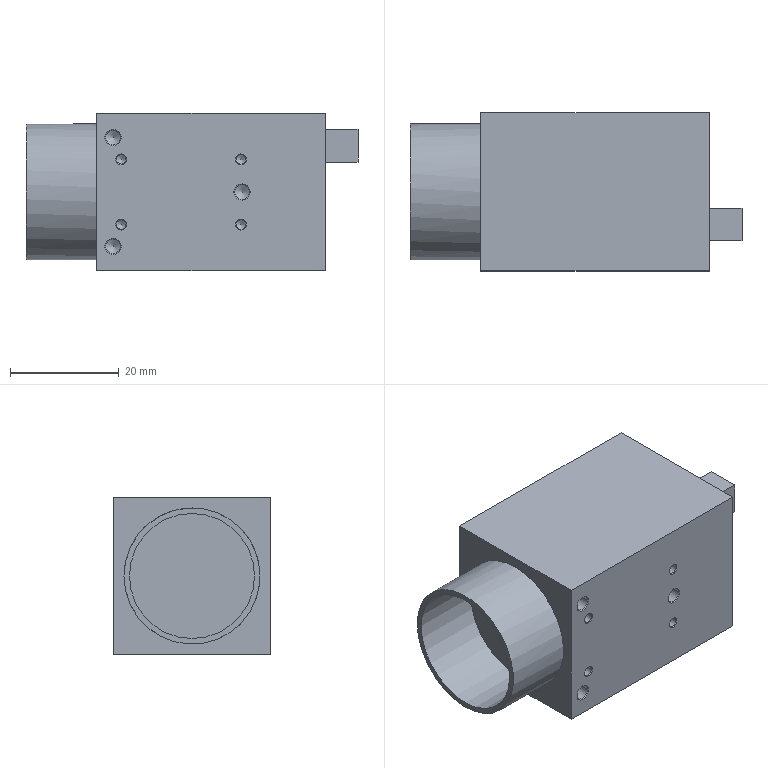Part | NX | features SIMPLE HOLE 7, SYMBOLIC_THREAD 7, DATUM_CSYS 6, SKETCH 5, EXTRUDE 4, HOLE PACKAGE 2 | 1 solid | 36 faces | box 61 x 29 x 29 mm | volume 36377 mm3 | cone 14 | plane 13 | cylinder 9 | commonest cylinder face diameters 1.75 x4 2.7 x3 23 x1 25 x1
STEP:
#1=CARTESIAN_POINT('',(16.,-14.5,-8.5));
#2=VERTEX_POINT('',#1);
#3=CARTESIAN_POINT('',(16.,-14.5,-10.));
#4=DIRECTION('',(0.,1.,0.));
#5=DIRECTION('',(0.,0.,1.));
#6=AXIS2_PLACEMENT_3D('',#3,#4,#5);
#7=CIRCLE('',#6,1.5);
#8=EDGE_CURVE('',#2,#2,#7,.T.);
#9=ORIENTED_EDGE('',*,*,#8,.T.);
#10=EDGE_LOOP('',(#9));
#11=FACE_BOUND('',#10,.T.);
#12=CARTESIAN_POINT('',(16.,-14.5,11.5));
#13=VERTEX_POINT('',#12);
#14=CARTESIAN_POINT('',(16.,-14.5,10.));
#15=DIRECTION('',(0.,1.,0.));
#16=DIRECTION('',(0.,0.,1.));
#17=AXIS2_PLACEMENT_3D('',#14,#15,#16);
#18=CIRCLE('',#17,1.5);
#19=EDGE_CURVE('',#13,#13,#18,.T.);
#20=ORIENTED_EDGE('',*,*,#19,.T.);
#21=EDGE_LOOP('',(#20));
#22=FACE_BOUND('',#21,.T.);
#23=CARTESIAN_POINT('',(39.7,-14.5,1.5));
#24=VERTEX_POINT('',#23);
#25=CARTESIAN_POINT('',(39.7,-14.5,0.));
#26=DIRECTION('',(0.,1.,0.));
#27=DIRECTION('',(0.,0.,1.));
#28=AXIS2_PLACEMENT_3D('',#25,#26,#27);
#29=CIRCLE('',#28,1.5);
#30=EDGE_CURVE('',#24,#24,#29,.T.);
#31=ORIENTED_EDGE('',*,*,#30,.T.);
#32=EDGE_LOOP('',(#31));
#33=FACE_BOUND('',#32,.T.);
#34=CARTESIAN_POINT('',(39.5,-14.5,-5.));
#35=VERTEX_POINT('',#34);
#36=CARTESIAN_POINT('',(39.5,-14.5,-6.));
#37=DIRECTION('',(0.,1.,0.));
#38=DIRECTION('',(0.,0.,1.));
#39=AXIS2_PLACEMENT_3D('',#36,#37,#38);
#40=CIRCLE('',#39,1.);
#41=EDGE_CURVE('',#35,#35,#40,.T.);
#42=ORIENTED_EDGE('',*,*,#41,.T.);
#43=EDGE_LOOP('',(#42));
#44=FACE_BOUND('',#43,.T.);
#45=CARTESIAN_POINT('',(39.5,-14.5,7.));
#46=VERTEX_POINT('',#45);
#47=CARTESIAN_POINT('',(39.5,-14.5,6.));
#48=DIRECTION('',(0.,1.,0.));
#49=DIRECTION('',(0.,0.,1.));
#50=AXIS2_PLACEMENT_3D('',#47,#48,#49);
#51=CIRCLE('',#50,1.);
#52=EDGE_CURVE('',#46,#46,#51,.T.);
#53=ORIENTED_EDGE('',*,*,#52,.T.);
#54=EDGE_LOOP('',(#53));
#55=FACE_BOUND('',#54,.T.);
#56=CARTESIAN_POINT('',(17.5,-14.5,-5.));
#57=VERTEX_POINT('',#56);
#58=CARTESIAN_POINT('',(17.5,-14.5,-6.));
#59=DIRECTION('',(0.,1.,0.));
#60=DIRECTION('',(0.,0.,1.));
#61=AXIS2_PLACEMENT_3D('',#58,#59,#60);
#62=CIRCLE('',#61,1.);
#63=EDGE_CURVE('',#57,#57,#62,.T.);
#64=ORIENTED_EDGE('',*,*,#63,.T.);
#65=EDGE_LOOP('',(#64));
#66=FACE_BOUND('',#65,.T.);
#67=CARTESIAN_POINT('',(17.5,-14.5,7.));
#68=VERTEX_POINT('',#67);
#69=CARTESIAN_POINT('',(17.5,-14.5,6.));
#70=DIRECTION('',(0.,1.,0.));
#71=DIRECTION('',(0.,0.,1.));
#72=AXIS2_PLACEMENT_3D('',#69,#70,#71);
#73=CIRCLE('',#72,1.);
#74=EDGE_CURVE('',#68,#68,#73,.T.);
#75=ORIENTED_EDGE('',*,*,#74,.T.);
#76=EDGE_LOOP('',(#75));
#77=FACE_BOUND('',#76,.T.);
#78=CARTESIAN_POINT('',(13.,-14.5,-14.5));
#79=VERTEX_POINT('',#78);
#80=CARTESIAN_POINT('',(13.,-14.5,14.5));
#81=VERTEX_POINT('',#80);
#82=CARTESIAN_POINT('',(13.,-14.5,-14.5));
#83=DIRECTION('',(0.,0.,1.));
#84=VECTOR('',#83,1000.);
#85=LINE('',#82,#84);
#86=EDGE_CURVE('',#79,#81,#85,.T.);
#87=ORIENTED_EDGE('',*,*,#86,.F.);
#88=CARTESIAN_POINT('',(55.,-14.5,-14.5));
#89=VERTEX_POINT('',#88);
#90=CARTESIAN_POINT('',(55.,-14.5,-14.5));
#91=DIRECTION('',(-1.,0.,0.));
#92=VECTOR('',#91,1000.);
#93=LINE('',#90,#92);
#94=EDGE_CURVE('',#89,#79,#93,.T.);
#95=ORIENTED_EDGE('',*,*,#94,.F.);
#96=CARTESIAN_POINT('',(55.,-14.5,14.5));
#97=VERTEX_POINT('',#96);
#98=CARTESIAN_POINT('',(55.,-14.5,14.5));
#99=DIRECTION('',(0.,0.,-1.));
#100=VECTOR('',#99,1000.);
#101=LINE('',#98,#100);
#102=EDGE_CURVE('',#97,#89,#101,.T.);
#103=ORIENTED_EDGE('',*,*,#102,.F.);
#104=CARTESIAN_POINT('',(55.,-14.5,14.5));
#105=DIRECTION('',(-1.,0.,0.));
#106=VECTOR('',#105,1000.);
#107=LINE('',#104,#106);
#108=EDGE_CURVE('',#97,#81,#107,.T.);
#109=ORIENTED_EDGE('',*,*,#108,.T.);
#110=EDGE_LOOP('',(#87,#95,#103,#109));
#111=FACE_BOUND('',#110,.T.);
#112=CARTESIAN_POINT('',(55.,-14.5,14.5));
#113=DIRECTION('',(0.,1.,0.));
#114=DIRECTION('',(0.,0.,1.));
#115=AXIS2_PLACEMENT_3D('',#112,#113,#114);
#116=PLANE('',#115);
#117=ADVANCED_FACE('',(#11,#22,#33,#44,#55,#66,#77,#111),#116,.F.);
#118=CARTESIAN_POINT('',(13.,14.5,-14.5));
#119=VERTEX_POINT('',#118);
#120=CARTESIAN_POINT('',(13.,14.5,-14.5));
#121=DIRECTION('',(0.,-1.,0.));
#122=VECTOR('',#121,1000.);
#123=LINE('',#120,#122);
#124=EDGE_CURVE('',#119,#79,#123,.T.);
#125=ORIENTED_EDGE('',*,*,#124,.F.);
#126=CARTESIAN_POINT('',(55.,14.5,-14.5));
#127=VERTEX_POINT('',#126);
#128=CARTESIAN_POINT('',(55.,14.5,-14.5));
#129=DIRECTION('',(-1.,0.,0.));
#130=VECTOR('',#129,1000.);
#131=LINE('',#128,#130);
#132=EDGE_CURVE('',#127,#119,#131,.T.);
#133=ORIENTED_EDGE('',*,*,#132,.F.);
#134=CARTESIAN_POINT('',(55.,-14.5,-14.5));
#135=DIRECTION('',(0.,1.,0.));
#136=VECTOR('',#135,1000.);
#137=LINE('',#134,#136);
#138=EDGE_CURVE('',#89,#127,#137,.T.);
#139=ORIENTED_EDGE('',*,*,#138,.F.);
#140=ORIENTED_EDGE('',*,*,#94,.T.);
#141=EDGE_LOOP('',(#125,#133,#139,#140));
#142=FACE_BOUND('',#141,.T.);
#143=CARTESIAN_POINT('',(55.,-14.5,-14.5));
#144=DIRECTION('',(0.,0.,1.));
#145=DIRECTION('',(1.,0.,0.));
#146=AXIS2_PLACEMENT_3D('',#143,#144,#145);
#147=PLANE('',#146);
#148=ADVANCED_FACE('',(#142),#147,.F.);
#149=CARTESIAN_POINT('',(13.,14.5,14.5));
#150=VERTEX_POINT('',#149);
#151=CARTESIAN_POINT('',(13.,14.5,14.5));
#152=DIRECTION('',(0.,0.,-1.));
#153=VECTOR('',#152,1000.);
#154=LINE('',#151,#153);
#155=EDGE_CURVE('',#150,#119,#154,.T.);
#156=ORIENTED_EDGE('',*,*,#155,.F.);
#157=CARTESIAN_POINT('',(55.,14.5,14.5));
#158=VERTEX_POINT('',#157);
#159=CARTESIAN_POINT('',(55.,14.5,14.5));
#160=DIRECTION('',(-1.,0.,0.));
#161=VECTOR('',#160,1000.);
#162=LINE('',#159,#161);
#163=EDGE_CURVE('',#158,#150,#162,.T.);
#164=ORIENTED_EDGE('',*,*,#163,.F.);
#165=CARTESIAN_POINT('',(55.,14.5,-14.5));
#166=DIRECTION('',(0.,0.,1.));
#167=VECTOR('',#166,1000.);
#168=LINE('',#165,#167);
#169=EDGE_CURVE('',#127,#158,#168,.T.);
#170=ORIENTED_EDGE('',*,*,#169,.F.);
#171=ORIENTED_EDGE('',*,*,#132,.T.);
#172=EDGE_LOOP('',(#156,#164,#170,#171));
#173=FACE_BOUND('',#172,.T.);
#174=CARTESIAN_POINT('',(55.,14.5,-14.5));
#175=DIRECTION('',(0.,-1.,0.));
#176=DIRECTION('',(0.,0.,-1.));
#177=AXIS2_PLACEMENT_3D('',#174,#175,#176);
#178=PLANE('',#177);
#179=ADVANCED_FACE('',(#173),#178,.F.);
#180=CARTESIAN_POINT('',(13.,-14.5,14.5));
#181=DIRECTION('',(0.,1.,0.));
#182=VECTOR('',#181,1000.);
#183=LINE('',#180,#182);
#184=EDGE_CURVE('',#81,#150,#183,.T.);
#185=ORIENTED_EDGE('',*,*,#184,.F.);
#186=ORIENTED_EDGE('',*,*,#108,.F.);
#187=CARTESIAN_POINT('',(55.,14.5,14.5));
#188=DIRECTION('',(0.,-1.,0.));
#189=VECTOR('',#188,1000.);
#190=LINE('',#187,#189);
#191=EDGE_CURVE('',#158,#97,#190,.T.);
#192=ORIENTED_EDGE('',*,*,#191,.F.);
#193=ORIENTED_EDGE('',*,*,#163,.T.);
#194=EDGE_LOOP('',(#185,#186,#192,#193));
#195=FACE_BOUND('',#194,.T.);
#196=CARTESIAN_POINT('',(55.,14.5,14.5));
#197=DIRECTION('',(0.,0.,-1.));
#198=DIRECTION('',(-1.,0.,0.));
#199=AXIS2_PLACEMENT_3D('',#196,#197,#198);
#200=PLANE('',#199);
#201=ADVANCED_FACE('',(#195),#200,.F.);
#202=CARTESIAN_POINT('',(55.,-9.,11.5));
#203=VERTEX_POINT('',#202);
#204=CARTESIAN_POINT('',(55.,-9.,5.5));
#205=VERTEX_POINT('',#204);
#206=CARTESIAN_POINT('',(55.,-9.,11.5));
#207=DIRECTION('',(0.,0.,-1.));
#208=VECTOR('',#207,1000.);
#209=LINE('',#206,#208);
#210=EDGE_CURVE('',#203,#205,#209,.T.);
#211=ORIENTED_EDGE('',*,*,#210,.F.);
#212=CARTESIAN_POINT('',(55.,-3.,11.5));
#213=VERTEX_POINT('',#212);
#214=CARTESIAN_POINT('',(55.,-3.,11.5));
#215=DIRECTION('',(0.,-1.,0.));
#216=VECTOR('',#215,1000.);
#217=LINE('',#214,#216);
#218=EDGE_CURVE('',#213,#203,#217,.T.);
#219=ORIENTED_EDGE('',*,*,#218,.F.);
#220=CARTESIAN_POINT('',(55.,-3.,5.5));
#221=VERTEX_POINT('',#220);
#222=CARTESIAN_POINT('',(55.,-3.,5.5));
#223=DIRECTION('',(0.,0.,1.));
#224=VECTOR('',#223,1000.);
#225=LINE('',#222,#224);
#226=EDGE_CURVE('',#221,#213,#225,.T.);
#227=ORIENTED_EDGE('',*,*,#226,.F.);
#228=CARTESIAN_POINT('',(55.,-9.,5.5));
#229=DIRECTION('',(0.,1.,0.));
#230=VECTOR('',#229,1000.);
#231=LINE('',#228,#230);
#232=EDGE_CURVE('',#205,#221,#231,.T.);
#233=ORIENTED_EDGE('',*,*,#232,.F.);
#234=EDGE_LOOP('',(#211,#219,#227,#233));
#235=FACE_BOUND('',#234,.T.);
#236=ORIENTED_EDGE('',*,*,#102,.T.);
#237=ORIENTED_EDGE('',*,*,#138,.T.);
#238=ORIENTED_EDGE('',*,*,#169,.T.);
#239=ORIENTED_EDGE('',*,*,#191,.T.);
#240=EDGE_LOOP('',(#236,#237,#238,#239));
#241=FACE_BOUND('',#240,.T.);
#242=CARTESIAN_POINT('',(55.,0.,0.));
#243=DIRECTION('',(1.,0.,0.));
#244=DIRECTION('',(0.,0.,-1.));
#245=AXIS2_PLACEMENT_3D('',#242,#243,#244);
#246=PLANE('',#245);
#247=ADVANCED_FACE('',(#235,#241),#246,.T.);
#248=CARTESIAN_POINT('',(16.,-9.5,-8.65));
#249=VERTEX_POINT('',#248);
#250=CARTESIAN_POINT('',(16.,-9.5,-10.));
#251=DIRECTION('',(0.,1.,0.));
#252=DIRECTION('',(0.,0.,1.));
#253=AXIS2_PLACEMENT_3D('',#250,#251,#252);
#254=CIRCLE('',#253,1.35);
#255=EDGE_CURVE('',#249,#249,#254,.F.);
#256=ORIENTED_EDGE('',*,*,#255,.T.);
#257=EDGE_LOOP('',(#256));
#258=FACE_BOUND('',#257,.T.);
#259=CARTESIAN_POINT('',(16.,-8.689,-10.));
#260=VERTEX_POINT('',#259);
#261=VERTEX_LOOP('',#260);
#262=FACE_BOUND('',#261,.T.);
#263=CARTESIAN_POINT('',(16.,-9.5,-10.));
#264=DIRECTION('',(0.,-1.,0.));
#265=DIRECTION('',(0.,0.,-1.));
#266=AXIS2_PLACEMENT_3D('',#263,#264,#265);
#267=CONICAL_SURFACE('',#266,1.35,1.03);
#268=ADVANCED_FACE('',(#258,#262),#267,.F.);
#269=CARTESIAN_POINT('',(16.,-14.35,-8.65));
#270=VERTEX_POINT('',#269);
#271=CARTESIAN_POINT('',(16.,-14.35,-10.));
#272=DIRECTION('',(0.,1.,0.));
#273=DIRECTION('',(0.,0.,1.));
#274=AXIS2_PLACEMENT_3D('',#271,#272,#273);
#275=CIRCLE('',#274,1.35);
#276=EDGE_CURVE('',#270,#270,#275,.F.);
#277=ORIENTED_EDGE('',*,*,#276,.T.);
#278=EDGE_LOOP('',(#277));
#279=FACE_BOUND('',#278,.T.);
#280=ORIENTED_EDGE('',*,*,#255,.F.);
#281=EDGE_LOOP('',(#280));
#282=FACE_BOUND('',#281,.T.);
#283=CARTESIAN_POINT('',(16.,-14.5,-10.));
#284=DIRECTION('',(0.,1.,0.));
#285=DIRECTION('',(0.,0.,1.));
#286=AXIS2_PLACEMENT_3D('',#283,#284,#285);
#287=CYLINDRICAL_SURFACE('',#286,1.35);
#288=ADVANCED_FACE('',(#279,#282),#287,.F.);
#289=ORIENTED_EDGE('',*,*,#276,.F.);
#290=EDGE_LOOP('',(#289));
#291=FACE_BOUND('',#290,.T.);
#292=ORIENTED_EDGE('',*,*,#8,.F.);
#293=EDGE_LOOP('',(#292));
#294=FACE_BOUND('',#293,.T.);
#295=CARTESIAN_POINT('',(16.,-14.5,-10.));
#296=DIRECTION('',(0.,-1.,0.));
#297=DIRECTION('',(0.,0.,-1.));
#298=AXIS2_PLACEMENT_3D('',#295,#296,#297);
#299=CONICAL_SURFACE('',#298,1.5,0.7854);
#300=ADVANCED_FACE('',(#291,#294),#299,.F.);
#301=CARTESIAN_POINT('',(16.,-9.5,11.35));
#302=VERTEX_POINT('',#301);
#303=CARTESIAN_POINT('',(16.,-9.5,10.));
#304=DIRECTION('',(0.,1.,0.));
#305=DIRECTION('',(0.,0.,1.));
#306=AXIS2_PLACEMENT_3D('',#303,#304,#305);
#307=CIRCLE('',#306,1.35);
#308=EDGE_CURVE('',#302,#302,#307,.F.);
#309=ORIENTED_EDGE('',*,*,#308,.T.);
#310=EDGE_LOOP('',(#309));
#311=FACE_BOUND('',#310,.T.);
#312=CARTESIAN_POINT('',(16.,-8.689,10.));
#313=VERTEX_POINT('',#312);
#314=VERTEX_LOOP('',#313);
#315=FACE_BOUND('',#314,.T.);
#316=CARTESIAN_POINT('',(16.,-9.5,10.));
#317=DIRECTION('',(0.,-1.,0.));
#318=DIRECTION('',(0.,0.,-1.));
#319=AXIS2_PLACEMENT_3D('',#316,#317,#318);
#320=CONICAL_SURFACE('',#319,1.35,1.03);
#321=ADVANCED_FACE('',(#311,#315),#320,.F.);
#322=CARTESIAN_POINT('',(16.,-14.35,11.35));
#323=VERTEX_POINT('',#322);
#324=CARTESIAN_POINT('',(16.,-14.35,10.));
#325=DIRECTION('',(0.,1.,0.));
#326=DIRECTION('',(0.,0.,1.));
#327=AXIS2_PLACEMENT_3D('',#324,#325,#326);
#328=CIRCLE('',#327,1.35);
#329=EDGE_CURVE('',#323,#323,#328,.F.);
#330=ORIENTED_EDGE('',*,*,#329,.T.);
#331=EDGE_LOOP('',(#330));
#332=FACE_BOUND('',#331,.T.);
#333=ORIENTED_EDGE('',*,*,#308,.F.);
#334=EDGE_LOOP('',(#333));
#335=FACE_BOUND('',#334,.T.);
#336=CARTESIAN_POINT('',(16.,-14.5,10.));
#337=DIRECTION('',(0.,1.,0.));
#338=DIRECTION('',(0.,0.,1.));
#339=AXIS2_PLACEMENT_3D('',#336,#337,#338);
#340=CYLINDRICAL_SURFACE('',#339,1.35);
#341=ADVANCED_FACE('',(#332,#335),#340,.F.);
#342=ORIENTED_EDGE('',*,*,#329,.F.);
#343=EDGE_LOOP('',(#342));
#344=FACE_BOUND('',#343,.T.);
#345=ORIENTED_EDGE('',*,*,#19,.F.);
#346=EDGE_LOOP('',(#345));
#347=FACE_BOUND('',#346,.T.);
#348=CARTESIAN_POINT('',(16.,-14.5,10.));
#349=DIRECTION('',(0.,-1.,0.));
#350=DIRECTION('',(0.,0.,-1.));
#351=AXIS2_PLACEMENT_3D('',#348,#349,#350);
#352=CONICAL_SURFACE('',#351,1.5,0.7854);
#353=ADVANCED_FACE('',(#344,#347),#352,.F.);
#354=CARTESIAN_POINT('',(39.7,-9.5,1.35));
#355=VERTEX_POINT('',#354);
#356=CARTESIAN_POINT('',(39.7,-9.5,0.));
#357=DIRECTION('',(0.,1.,0.));
#358=DIRECTION('',(0.,0.,1.));
#359=AXIS2_PLACEMENT_3D('',#356,#357,#358);
#360=CIRCLE('',#359,1.35);
#361=EDGE_CURVE('',#355,#355,#360,.F.);
#362=ORIENTED_EDGE('',*,*,#361,.T.);
#363=EDGE_LOOP('',(#362));
#364=FACE_BOUND('',#363,.T.);
#365=CARTESIAN_POINT('',(39.7,-8.689,0.));
#366=VERTEX_POINT('',#365);
#367=VERTEX_LOOP('',#366);
#368=FACE_BOUND('',#367,.T.);
#369=CARTESIAN_POINT('',(39.7,-9.5,0.));
#370=DIRECTION('',(0.,-1.,0.));
#371=DIRECTION('',(0.,0.,-1.));
#372=AXIS2_PLACEMENT_3D('',#369,#370,#371);
#373=CONICAL_SURFACE('',#372,1.35,1.03);
#374=ADVANCED_FACE('',(#364,#368),#373,.F.);
#375=CARTESIAN_POINT('',(39.7,-14.35,1.35));
#376=VERTEX_POINT('',#375);
#377=CARTESIAN_POINT('',(39.7,-14.35,0.));
#378=DIRECTION('',(0.,1.,0.));
#379=DIRECTION('',(0.,0.,1.));
#380=AXIS2_PLACEMENT_3D('',#377,#378,#379);
#381=CIRCLE('',#380,1.35);
#382=EDGE_CURVE('',#376,#376,#381,.F.);
#383=ORIENTED_EDGE('',*,*,#382,.T.);
#384=EDGE_LOOP('',(#383));
#385=FACE_BOUND('',#384,.T.);
#386=ORIENTED_EDGE('',*,*,#361,.F.);
#387=EDGE_LOOP('',(#386));
#388=FACE_BOUND('',#387,.T.);
#389=CARTESIAN_POINT('',(39.7,-14.5,0.));
#390=DIRECTION('',(0.,1.,0.));
#391=DIRECTION('',(0.,0.,1.));
#392=AXIS2_PLACEMENT_3D('',#389,#390,#391);
#393=CYLINDRICAL_SURFACE('',#392,1.35);
#394=ADVANCED_FACE('',(#385,#388),#393,.F.);
#395=ORIENTED_EDGE('',*,*,#382,.F.);
#396=EDGE_LOOP('',(#395));
#397=FACE_BOUND('',#396,.T.);
#398=ORIENTED_EDGE('',*,*,#30,.F.);
#399=EDGE_LOOP('',(#398));
#400=FACE_BOUND('',#399,.T.);
#401=CARTESIAN_POINT('',(39.7,-14.5,0.));
#402=DIRECTION('',(0.,-1.,0.));
#403=DIRECTION('',(0.,0.,-1.));
#404=AXIS2_PLACEMENT_3D('',#401,#402,#403);
#405=CONICAL_SURFACE('',#404,1.5,0.7854);
#406=ADVANCED_FACE('',(#397,#400),#405,.F.);
#407=CARTESIAN_POINT('',(39.5,-9.5,-5.125));
#408=VERTEX_POINT('',#407);
#409=CARTESIAN_POINT('',(39.5,-9.5,-6.));
#410=DIRECTION('',(0.,1.,0.));
#411=DIRECTION('',(0.,0.,1.));
#412=AXIS2_PLACEMENT_3D('',#409,#410,#411);
#413=CIRCLE('',#412,0.875);
#414=EDGE_CURVE('',#408,#408,#413,.F.);
#415=ORIENTED_EDGE('',*,*,#414,.T.);
#416=EDGE_LOOP('',(#415));
#417=FACE_BOUND('',#416,.T.);
#418=CARTESIAN_POINT('',(39.5,-8.974,-6.));
#419=VERTEX_POINT('',#418);
#420=VERTEX_LOOP('',#419);
#421=FACE_BOUND('',#420,.T.);
#422=CARTESIAN_POINT('',(39.5,-9.5,-6.));
#423=DIRECTION('',(0.,-1.,0.));
#424=DIRECTION('',(0.,0.,-1.));
#425=AXIS2_PLACEMENT_3D('',#422,#423,#424);
#426=CONICAL_SURFACE('',#425,0.875,1.03);
#427=ADVANCED_FACE('',(#417,#421),#426,.F.);
#428=CARTESIAN_POINT('',(39.5,-14.375,-5.125));
#429=VERTEX_POINT('',#428);
#430=CARTESIAN_POINT('',(39.5,-14.375,-6.));
#431=DIRECTION('',(0.,1.,0.));
#432=DIRECTION('',(0.,0.,1.));
#433=AXIS2_PLACEMENT_3D('',#430,#431,#432);
#434=CIRCLE('',#433,0.875);
#435=EDGE_CURVE('',#429,#429,#434,.F.);
#436=ORIENTED_EDGE('',*,*,#435,.T.);
#437=EDGE_LOOP('',(#436));
#438=FACE_BOUND('',#437,.T.);
#439=ORIENTED_EDGE('',*,*,#414,.F.);
#440=EDGE_LOOP('',(#439));
#441=FACE_BOUND('',#440,.T.);
#442=CARTESIAN_POINT('',(39.5,-14.5,-6.));
#443=DIRECTION('',(0.,1.,0.));
#444=DIRECTION('',(0.,0.,1.));
#445=AXIS2_PLACEMENT_3D('',#442,#443,#444);
#446=CYLINDRICAL_SURFACE('',#445,0.875);
#447=ADVANCED_FACE('',(#438,#441),#446,.F.);
#448=ORIENTED_EDGE('',*,*,#435,.F.);
#449=EDGE_LOOP('',(#448));
#450=FACE_BOUND('',#449,.T.);
#451=ORIENTED_EDGE('',*,*,#41,.F.);
#452=EDGE_LOOP('',(#451));
#453=FACE_BOUND('',#452,.T.);
#454=CARTESIAN_POINT('',(39.5,-14.5,-6.));
#455=DIRECTION('',(0.,-1.,0.));
#456=DIRECTION('',(0.,0.,-1.));
#457=AXIS2_PLACEMENT_3D('',#454,#455,#456);
#458=CONICAL_SURFACE('',#457,1.,0.7854);
#459=ADVANCED_FACE('',(#450,#453),#458,.F.);
#460=CARTESIAN_POINT('',(39.5,-9.5,6.875));
#461=VERTEX_POINT('',#460);
#462=CARTESIAN_POINT('',(39.5,-9.5,6.));
#463=DIRECTION('',(0.,1.,0.));
#464=DIRECTION('',(0.,0.,1.));
#465=AXIS2_PLACEMENT_3D('',#462,#463,#464);
#466=CIRCLE('',#465,0.875);
#467=EDGE_CURVE('',#461,#461,#466,.F.);
#468=ORIENTED_EDGE('',*,*,#467,.T.);
#469=EDGE_LOOP('',(#468));
#470=FACE_BOUND('',#469,.T.);
#471=CARTESIAN_POINT('',(39.5,-8.974,6.));
#472=VERTEX_POINT('',#471);
#473=VERTEX_LOOP('',#472);
#474=FACE_BOUND('',#473,.T.);
#475=CARTESIAN_POINT('',(39.5,-9.5,6.));
#476=DIRECTION('',(0.,-1.,0.));
#477=DIRECTION('',(0.,0.,-1.));
#478=AXIS2_PLACEMENT_3D('',#475,#476,#477);
#479=CONICAL_SURFACE('',#478,0.875,1.03);
#480=ADVANCED_FACE('',(#470,#474),#479,.F.);
#481=CARTESIAN_POINT('',(39.5,-14.375,6.875));
#482=VERTEX_POINT('',#481);
#483=CARTESIAN_POINT('',(39.5,-14.375,6.));
#484=DIRECTION('',(0.,1.,0.));
#485=DIRECTION('',(0.,0.,1.));
#486=AXIS2_PLACEMENT_3D('',#483,#484,#485);
#487=CIRCLE('',#486,0.875);
#488=EDGE_CURVE('',#482,#482,#487,.F.);
#489=ORIENTED_EDGE('',*,*,#488,.T.);
#490=EDGE_LOOP('',(#489));
#491=FACE_BOUND('',#490,.T.);
#492=ORIENTED_EDGE('',*,*,#467,.F.);
#493=EDGE_LOOP('',(#492));
#494=FACE_BOUND('',#493,.T.);
#495=CARTESIAN_POINT('',(39.5,-14.5,6.));
#496=DIRECTION('',(0.,1.,0.));
#497=DIRECTION('',(0.,0.,1.));
#498=AXIS2_PLACEMENT_3D('',#495,#496,#497);
#499=CYLINDRICAL_SURFACE('',#498,0.875);
#500=ADVANCED_FACE('',(#491,#494),#499,.F.);
#501=ORIENTED_EDGE('',*,*,#488,.F.);
#502=EDGE_LOOP('',(#501));
#503=FACE_BOUND('',#502,.T.);
#504=ORIENTED_EDGE('',*,*,#52,.F.);
#505=EDGE_LOOP('',(#504));
#506=FACE_BOUND('',#505,.T.);
#507=CARTESIAN_POINT('',(39.5,-14.5,6.));
#508=DIRECTION('',(0.,-1.,0.));
#509=DIRECTION('',(0.,0.,-1.));
#510=AXIS2_PLACEMENT_3D('',#507,#508,#509);
#511=CONICAL_SURFACE('',#510,1.,0.7854);
#512=ADVANCED_FACE('',(#503,#506),#511,.F.);
#513=CARTESIAN_POINT('',(17.5,-9.5,-5.125));
#514=VERTEX_POINT('',#513);
#515=CARTESIAN_POINT('',(17.5,-9.5,-6.));
#516=DIRECTION('',(0.,1.,0.));
#517=DIRECTION('',(0.,0.,1.));
#518=AXIS2_PLACEMENT_3D('',#515,#516,#517);
#519=CIRCLE('',#518,0.875);
#520=EDGE_CURVE('',#514,#514,#519,.F.);
#521=ORIENTED_EDGE('',*,*,#520,.T.);
#522=EDGE_LOOP('',(#521));
#523=FACE_BOUND('',#522,.T.);
#524=CARTESIAN_POINT('',(17.5,-8.974,-6.));
#525=VERTEX_POINT('',#524);
#526=VERTEX_LOOP('',#525);
#527=FACE_BOUND('',#526,.T.);
#528=CARTESIAN_POINT('',(17.5,-9.5,-6.));
#529=DIRECTION('',(0.,-1.,0.));
#530=DIRECTION('',(0.,0.,-1.));
#531=AXIS2_PLACEMENT_3D('',#528,#529,#530);
#532=CONICAL_SURFACE('',#531,0.875,1.03);
#533=ADVANCED_FACE('',(#523,#527),#532,.F.);
#534=CARTESIAN_POINT('',(17.5,-14.375,-5.125));
#535=VERTEX_POINT('',#534);
#536=CARTESIAN_POINT('',(17.5,-14.375,-6.));
#537=DIRECTION('',(0.,1.,0.));
#538=DIRECTION('',(0.,0.,1.));
#539=AXIS2_PLACEMENT_3D('',#536,#537,#538);
#540=CIRCLE('',#539,0.875);
#541=EDGE_CURVE('',#535,#535,#540,.F.);
#542=ORIENTED_EDGE('',*,*,#541,.T.);
#543=EDGE_LOOP('',(#542));
#544=FACE_BOUND('',#543,.T.);
#545=ORIENTED_EDGE('',*,*,#520,.F.);
#546=EDGE_LOOP('',(#545));
#547=FACE_BOUND('',#546,.T.);
#548=CARTESIAN_POINT('',(17.5,-14.5,-6.));
#549=DIRECTION('',(0.,1.,0.));
#550=DIRECTION('',(0.,0.,1.));
#551=AXIS2_PLACEMENT_3D('',#548,#549,#550);
#552=CYLINDRICAL_SURFACE('',#551,0.875);
#553=ADVANCED_FACE('',(#544,#547),#552,.F.);
#554=ORIENTED_EDGE('',*,*,#541,.F.);
#555=EDGE_LOOP('',(#554));
#556=FACE_BOUND('',#555,.T.);
#557=ORIENTED_EDGE('',*,*,#63,.F.);
#558=EDGE_LOOP('',(#557));
#559=FACE_BOUND('',#558,.T.);
#560=CARTESIAN_POINT('',(17.5,-14.5,-6.));
#561=DIRECTION('',(0.,-1.,0.));
#562=DIRECTION('',(0.,0.,-1.));
#563=AXIS2_PLACEMENT_3D('',#560,#561,#562);
#564=CONICAL_SURFACE('',#563,1.,0.7854);
#565=ADVANCED_FACE('',(#556,#559),#564,.F.);
#566=CARTESIAN_POINT('',(17.5,-9.5,6.875));
#567=VERTEX_POINT('',#566);
#568=CARTESIAN_POINT('',(17.5,-9.5,6.));
#569=DIRECTION('',(0.,1.,0.));
#570=DIRECTION('',(0.,0.,1.));
#571=AXIS2_PLACEMENT_3D('',#568,#569,#570);
#572=CIRCLE('',#571,0.875);
#573=EDGE_CURVE('',#567,#567,#572,.F.);
#574=ORIENTED_EDGE('',*,*,#573,.T.);
#575=EDGE_LOOP('',(#574));
#576=FACE_BOUND('',#575,.T.);
#577=CARTESIAN_POINT('',(17.5,-8.974,6.));
#578=VERTEX_POINT('',#577);
#579=VERTEX_LOOP('',#578);
#580=FACE_BOUND('',#579,.T.);
#581=CARTESIAN_POINT('',(17.5,-9.5,6.));
#582=DIRECTION('',(0.,-1.,0.));
#583=DIRECTION('',(0.,0.,-1.));
#584=AXIS2_PLACEMENT_3D('',#581,#582,#583);
#585=CONICAL_SURFACE('',#584,0.875,1.03);
#586=ADVANCED_FACE('',(#576,#580),#585,.F.);
#587=CARTESIAN_POINT('',(17.5,-14.375,6.875));
#588=VERTEX_POINT('',#587);
#589=CARTESIAN_POINT('',(17.5,-14.375,6.));
#590=DIRECTION('',(0.,1.,0.));
#591=DIRECTION('',(0.,0.,1.));
#592=AXIS2_PLACEMENT_3D('',#589,#590,#591);
#593=CIRCLE('',#592,0.875);
#594=EDGE_CURVE('',#588,#588,#593,.F.);
#595=ORIENTED_EDGE('',*,*,#594,.T.);
#596=EDGE_LOOP('',(#595));
#597=FACE_BOUND('',#596,.T.);
#598=ORIENTED_EDGE('',*,*,#573,.F.);
#599=EDGE_LOOP('',(#598));
#600=FACE_BOUND('',#599,.T.);
#601=CARTESIAN_POINT('',(17.5,-14.5,6.));
#602=DIRECTION('',(0.,1.,0.));
#603=DIRECTION('',(0.,0.,1.));
#604=AXIS2_PLACEMENT_3D('',#601,#602,#603);
#605=CYLINDRICAL_SURFACE('',#604,0.875);
#606=ADVANCED_FACE('',(#597,#600),#605,.F.);
#607=ORIENTED_EDGE('',*,*,#594,.F.);
#608=EDGE_LOOP('',(#607));
#609=FACE_BOUND('',#608,.T.);
#610=ORIENTED_EDGE('',*,*,#74,.F.);
#611=EDGE_LOOP('',(#610));
#612=FACE_BOUND('',#611,.T.);
#613=CARTESIAN_POINT('',(17.5,-14.5,6.));
#614=DIRECTION('',(0.,-1.,0.));
#615=DIRECTION('',(0.,0.,-1.));
#616=AXIS2_PLACEMENT_3D('',#613,#614,#615);
#617=CONICAL_SURFACE('',#616,1.,0.7854);
#618=ADVANCED_FACE('',(#609,#612),#617,.F.);
#619=CARTESIAN_POINT('',(13.,0.,12.5));
#620=VERTEX_POINT('',#619);
#621=CARTESIAN_POINT('',(13.,0.,0.));
#622=DIRECTION('',(-1.,0.,0.));
#623=DIRECTION('',(0.,0.,1.));
#624=AXIS2_PLACEMENT_3D('',#621,#622,#623);
#625=CIRCLE('',#624,12.5);
#626=EDGE_CURVE('',#620,#620,#625,.F.);
#627=ORIENTED_EDGE('',*,*,#626,.T.);
#628=EDGE_LOOP('',(#627));
#629=FACE_BOUND('',#628,.T.);
#630=ORIENTED_EDGE('',*,*,#86,.T.);
#631=ORIENTED_EDGE('',*,*,#184,.T.);
#632=ORIENTED_EDGE('',*,*,#155,.T.);
#633=ORIENTED_EDGE('',*,*,#124,.T.);
#634=EDGE_LOOP('',(#630,#631,#632,#633));
#635=FACE_BOUND('',#634,.T.);
#636=CARTESIAN_POINT('',(13.,0.,0.));
#637=DIRECTION('',(-1.,0.,0.));
#638=DIRECTION('',(0.,0.,1.));
#639=AXIS2_PLACEMENT_3D('',#636,#637,#638);
#640=PLANE('',#639);
#641=ADVANCED_FACE('',(#629,#635),#640,.T.);
#642=ORIENTED_EDGE('',*,*,#626,.F.);
#643=EDGE_LOOP('',(#642));
#644=FACE_BOUND('',#643,.T.);
#645=CARTESIAN_POINT('',(0.,12.5,0.));
#646=VERTEX_POINT('',#645);
#647=CARTESIAN_POINT('',(0.,0.,0.));
#648=DIRECTION('',(1.,0.,0.));
#649=DIRECTION('',(0.,1.,0.));
#650=AXIS2_PLACEMENT_3D('',#647,#648,#649);
#651=CIRCLE('',#650,12.5);
#652=EDGE_CURVE('',#646,#646,#651,.T.);
#653=ORIENTED_EDGE('',*,*,#652,.T.);
#654=EDGE_LOOP('',(#653));
#655=FACE_BOUND('',#654,.T.);
#656=CARTESIAN_POINT('',(0.,0.,0.));
#657=DIRECTION('',(1.,0.,0.));
#658=DIRECTION('',(0.,0.,-1.));
#659=AXIS2_PLACEMENT_3D('',#656,#657,#658);
#660=CYLINDRICAL_SURFACE('',#659,12.5);
#661=ADVANCED_FACE('',(#644,#655),#660,.T.);
#662=CARTESIAN_POINT('',(13.,0.,11.5));
#663=VERTEX_POINT('',#662);
#664=CARTESIAN_POINT('',(13.,0.,0.));
#665=DIRECTION('',(-1.,0.,0.));
#666=DIRECTION('',(0.,0.,1.));
#667=AXIS2_PLACEMENT_3D('',#664,#665,#666);
#668=CIRCLE('',#667,11.5);
#669=EDGE_CURVE('',#663,#663,#668,.F.);
#670=ORIENTED_EDGE('',*,*,#669,.T.);
#671=EDGE_LOOP('',(#670));
#672=FACE_BOUND('',#671,.T.);
#673=CARTESIAN_POINT('',(0.,0.,-11.5));
#674=VERTEX_POINT('',#673);
#675=CARTESIAN_POINT('',(0.,0.,0.));
#676=DIRECTION('',(1.,0.,0.));
#677=DIRECTION('',(0.,0.,-1.));
#678=AXIS2_PLACEMENT_3D('',#675,#676,#677);
#679=CIRCLE('',#678,11.5);
#680=EDGE_CURVE('',#674,#674,#679,.T.);
#681=ORIENTED_EDGE('',*,*,#680,.F.);
#682=EDGE_LOOP('',(#681));
#683=FACE_BOUND('',#682,.T.);
#684=CARTESIAN_POINT('',(0.,0.,0.));
#685=DIRECTION('',(1.,0.,0.));
#686=DIRECTION('',(0.,0.,-1.));
#687=AXIS2_PLACEMENT_3D('',#684,#685,#686);
#688=CYLINDRICAL_SURFACE('',#687,11.5);
#689=ADVANCED_FACE('',(#672,#683),#688,.F.);
#690=ORIENTED_EDGE('',*,*,#680,.T.);
#691=EDGE_LOOP('',(#690));
#692=FACE_BOUND('',#691,.T.);
#693=ORIENTED_EDGE('',*,*,#652,.F.);
#694=EDGE_LOOP('',(#693));
#695=FACE_BOUND('',#694,.T.);
#696=CARTESIAN_POINT('',(0.,0.,0.));
#697=DIRECTION('',(-1.,0.,0.));
#698=DIRECTION('',(0.,0.,1.));
#699=AXIS2_PLACEMENT_3D('',#696,#697,#698);
#700=PLANE('',#699);
#701=ADVANCED_FACE('',(#692,#695),#700,.T.);
#702=ORIENTED_EDGE('',*,*,#669,.F.);
#703=EDGE_LOOP('',(#702));
#704=FACE_BOUND('',#703,.T.);
#705=CARTESIAN_POINT('',(13.,0.,0.));
#706=DIRECTION('',(-1.,0.,0.));
#707=DIRECTION('',(0.,0.,1.));
#708=AXIS2_PLACEMENT_3D('',#705,#706,#707);
#709=PLANE('',#708);
#710=ADVANCED_FACE('',(#704),#709,.T.);
#711=ORIENTED_EDGE('',*,*,#210,.T.);
#712=CARTESIAN_POINT('',(61.,-9.,5.5));
#713=VERTEX_POINT('',#712);
#714=CARTESIAN_POINT('',(61.,-9.,5.5));
#715=DIRECTION('',(-1.,0.,0.));
#716=VECTOR('',#715,1000.);
#717=LINE('',#714,#716);
#718=EDGE_CURVE('',#713,#205,#717,.T.);
#719=ORIENTED_EDGE('',*,*,#718,.F.);
#720=CARTESIAN_POINT('',(61.,-9.,11.5));
#721=VERTEX_POINT('',#720);
#722=CARTESIAN_POINT('',(61.,-9.,11.5));
#723=DIRECTION('',(0.,0.,-1.));
#724=VECTOR('',#723,1000.);
#725=LINE('',#722,#724);
#726=EDGE_CURVE('',#721,#713,#725,.T.);
#727=ORIENTED_EDGE('',*,*,#726,.F.);
#728=CARTESIAN_POINT('',(61.,-9.,11.5));
#729=DIRECTION('',(-1.,0.,0.));
#730=VECTOR('',#729,1000.);
#731=LINE('',#728,#730);
#732=EDGE_CURVE('',#721,#203,#731,.T.);
#733=ORIENTED_EDGE('',*,*,#732,.T.);
#734=EDGE_LOOP('',(#711,#719,#727,#733));
#735=FACE_BOUND('',#734,.T.);
#736=CARTESIAN_POINT('',(61.,-9.,11.5));
#737=DIRECTION('',(0.,1.,0.));
#738=DIRECTION('',(0.,0.,1.));
#739=AXIS2_PLACEMENT_3D('',#736,#737,#738);
#740=PLANE('',#739);
#741=ADVANCED_FACE('',(#735),#740,.F.);
#742=ORIENTED_EDGE('',*,*,#232,.T.);
#743=CARTESIAN_POINT('',(61.,-3.,5.5));
#744=VERTEX_POINT('',#743);
#745=CARTESIAN_POINT('',(61.,-3.,5.5));
#746=DIRECTION('',(-1.,0.,0.));
#747=VECTOR('',#746,1000.);
#748=LINE('',#745,#747);
#749=EDGE_CURVE('',#744,#221,#748,.T.);
#750=ORIENTED_EDGE('',*,*,#749,.F.);
#751=CARTESIAN_POINT('',(61.,-9.,5.5));
#752=DIRECTION('',(0.,1.,0.));
#753=VECTOR('',#752,1000.);
#754=LINE('',#751,#753);
#755=EDGE_CURVE('',#713,#744,#754,.T.);
#756=ORIENTED_EDGE('',*,*,#755,.F.);
#757=ORIENTED_EDGE('',*,*,#718,.T.);
#758=EDGE_LOOP('',(#742,#750,#756,#757));
#759=FACE_BOUND('',#758,.T.);
#760=CARTESIAN_POINT('',(61.,-9.,5.5));
#761=DIRECTION('',(0.,0.,1.));
#762=DIRECTION('',(1.,0.,0.));
#763=AXIS2_PLACEMENT_3D('',#760,#761,#762);
#764=PLANE('',#763);
#765=ADVANCED_FACE('',(#759),#764,.F.);
#766=ORIENTED_EDGE('',*,*,#226,.T.);
#767=CARTESIAN_POINT('',(61.,-3.,11.5));
#768=VERTEX_POINT('',#767);
#769=CARTESIAN_POINT('',(61.,-3.,11.5));
#770=DIRECTION('',(-1.,0.,0.));
#771=VECTOR('',#770,1000.);
#772=LINE('',#769,#771);
#773=EDGE_CURVE('',#768,#213,#772,.T.);
#774=ORIENTED_EDGE('',*,*,#773,.F.);
#775=CARTESIAN_POINT('',(61.,-3.,5.5));
#776=DIRECTION('',(0.,0.,1.));
#777=VECTOR('',#776,1000.);
#778=LINE('',#775,#777);
#779=EDGE_CURVE('',#744,#768,#778,.T.);
#780=ORIENTED_EDGE('',*,*,#779,.F.);
#781=ORIENTED_EDGE('',*,*,#749,.T.);
#782=EDGE_LOOP('',(#766,#774,#780,#781));
#783=FACE_BOUND('',#782,.T.);
#784=CARTESIAN_POINT('',(61.,-3.,5.5));
#785=DIRECTION('',(0.,-1.,0.));
#786=DIRECTION('',(0.,0.,-1.));
#787=AXIS2_PLACEMENT_3D('',#784,#785,#786);
#788=PLANE('',#787);
#789=ADVANCED_FACE('',(#783),#788,.F.);
#790=ORIENTED_EDGE('',*,*,#218,.T.);
#791=ORIENTED_EDGE('',*,*,#732,.F.);
#792=CARTESIAN_POINT('',(61.,-3.,11.5));
#793=DIRECTION('',(0.,-1.,0.));
#794=VECTOR('',#793,1000.);
#795=LINE('',#792,#794);
#796=EDGE_CURVE('',#768,#721,#795,.T.);
#797=ORIENTED_EDGE('',*,*,#796,.F.);
#798=ORIENTED_EDGE('',*,*,#773,.T.);
#799=EDGE_LOOP('',(#790,#791,#797,#798));
#800=FACE_BOUND('',#799,.T.);
#801=CARTESIAN_POINT('',(61.,-3.,11.5));
#802=DIRECTION('',(0.,0.,-1.));
#803=DIRECTION('',(-1.,0.,0.));
#804=AXIS2_PLACEMENT_3D('',#801,#802,#803);
#805=PLANE('',#804);
#806=ADVANCED_FACE('',(#800),#805,.F.);
#807=ORIENTED_EDGE('',*,*,#726,.T.);
#808=ORIENTED_EDGE('',*,*,#755,.T.);
#809=ORIENTED_EDGE('',*,*,#779,.T.);
#810=ORIENTED_EDGE('',*,*,#796,.T.);
#811=EDGE_LOOP('',(#807,#808,#809,#810));
#812=FACE_BOUND('',#811,.T.);
#813=CARTESIAN_POINT('',(61.,0.,0.));
#814=DIRECTION('',(1.,0.,0.));
#815=DIRECTION('',(0.,0.,-1.));
#816=AXIS2_PLACEMENT_3D('',#813,#814,#815);
#817=PLANE('',#816);
#818=ADVANCED_FACE('',(#812),#817,.T.);
#819=CLOSED_SHELL('',(#117,#148,#179,#201,#247,#268,#288,#300,#321,#341,#353,#374,#394,#406,#427,#447,#459,#480,#500,#512,#533,#553,#565,#586,#606,#618,#641,#661,#689,#701,#710,#741,#765,#789,#806,#818));
#820=MANIFOLD_SOLID_BREP('',#819);
#821=(LENGTH_UNIT()NAMED_UNIT(*)SI_UNIT(.MILLI.,.METRE.));
#822=UNCERTAINTY_MEASURE_WITH_UNIT(LENGTH_MEASURE(0.00001),#821,'','');
#823=(NAMED_UNIT(*)PLANE_ANGLE_UNIT()SI_UNIT($,.RADIAN.));
#824=(NAMED_UNIT(*)SI_UNIT($,.STERADIAN.)SOLID_ANGLE_UNIT());
#825=(GEOMETRIC_REPRESENTATION_CONTEXT(3)GLOBAL_UNCERTAINTY_ASSIGNED_CONTEXT((#822))GLOBAL_UNIT_ASSIGNED_CONTEXT((#821,#823,#824))REPRESENTATION_CONTEXT('',''));
#826=ADVANCED_BREP_SHAPE_REPRESENTATION('',(#820),#825);